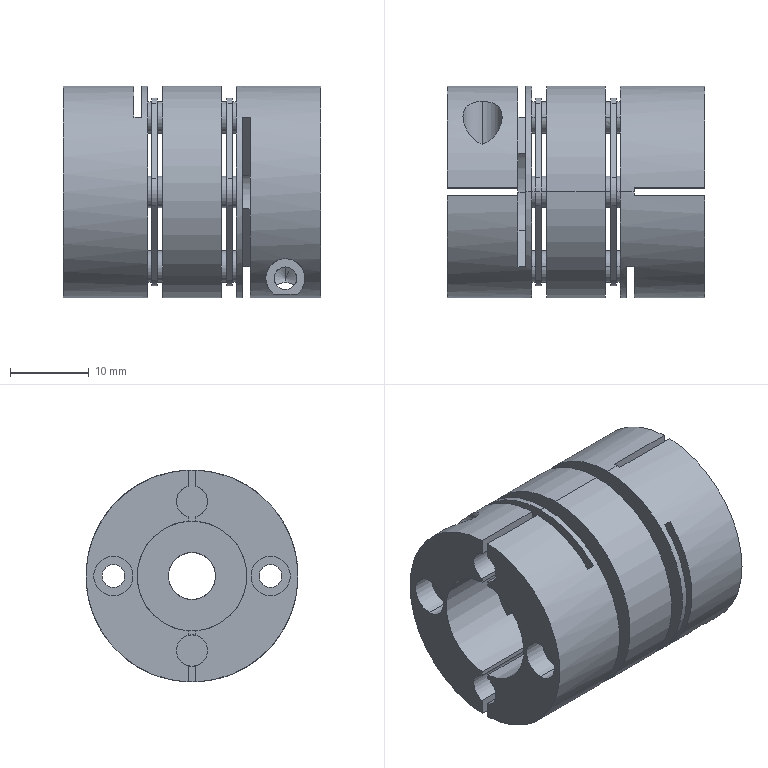Part | STEP file | double-diaphragm coupling LC-A-025DA-06B-14B-T001 | 1 solid | 150 faces | box 32.8 x 27 x 27 mm | volume 11316 mm3 | cylinder 84 | plane 58 | cone 8 | commonest cylinder face diameters 4 x22 5 x21 2.9 x16 17 x12 27 x6 2.05 x3